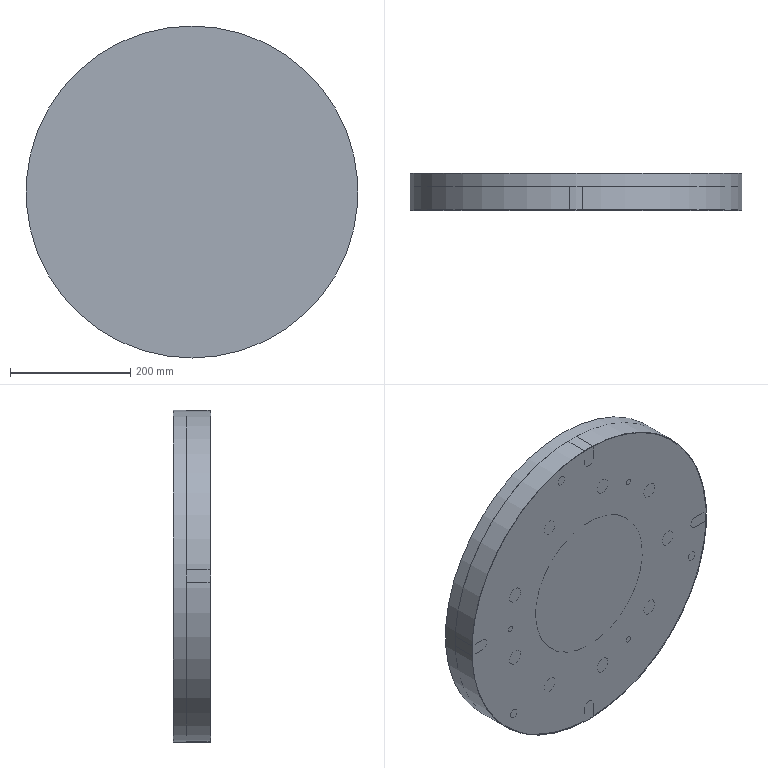CAM job | NX | 3-axis milling, drilling | part box 552 x 62 x 552 mm
Tools:
number,name,description,diameter,corner_radius,flute_length,length,flutes
1,点窝,Drilling Tool,3.0,0.0,35.0,50.0,2
2,D18,Milling Tool-5 Parameters,18.0,0.0,50.0,75.0,2
3,D8,Milling Tool-5 Parameters,8.0,0.0,50.0,75.0,2
0,D9,Drilling Tool,9.0,0.0,35.0,50.0,2
Operations:
program,operation,operation_type,tool,method,geometry_group,spindle_rpm,surface_speed,feed_per_tooth,feed_cut,feed_plunge,cut_length_mm,path_length_mm,cut_time_min,machine_time_min
A1,点窝,Operation,点窝,DRILL_METHOD,WORKPIECE,0.0,0.0,0.0,80.0,0.0,510.0,2868.125,6.375,6.611
A1,DRILLING,Operation,D9,DRILL_METHOD,WORKPIECE,900.0,25.0,0.0444,80.0,0.0,699.335,2471.081,8.742,8.919
A2,9-28槽_COPY,CavityMilling,D18,METHOD,WORKPIECE,900.0,50.0,0.0333,60.0,100.0,135.099,191.559,2.252,2.257
A3,CAVITY_MILL,CavityMilling,D18,METHOD,WORKPIECE,900.0,50.0,0.0333,60.0,100.0,3597.28,3764.213,59.955,59.971
NC_PROGRAM,CAVITY_MILL_COPY,CavityMilling,D18,METHOD,WORKPIECE,900.0,50.0,0.0333,60.0,100.0,119.697,277.697,1.995,2.011
A5,铣键槽,CavityMilling,D8,METHOD,WORKPIECE,2666.0,67.0,0.0169,90.0,100.0,441.3,542.243,4.903,4.913
A6,CAVITY_MILL_1,CavityMilling,D8,METHOD,WORKPIECE,900.0,22.0,0.0444,80.0,100.0,3273.52,4873.007,40.919,41.079